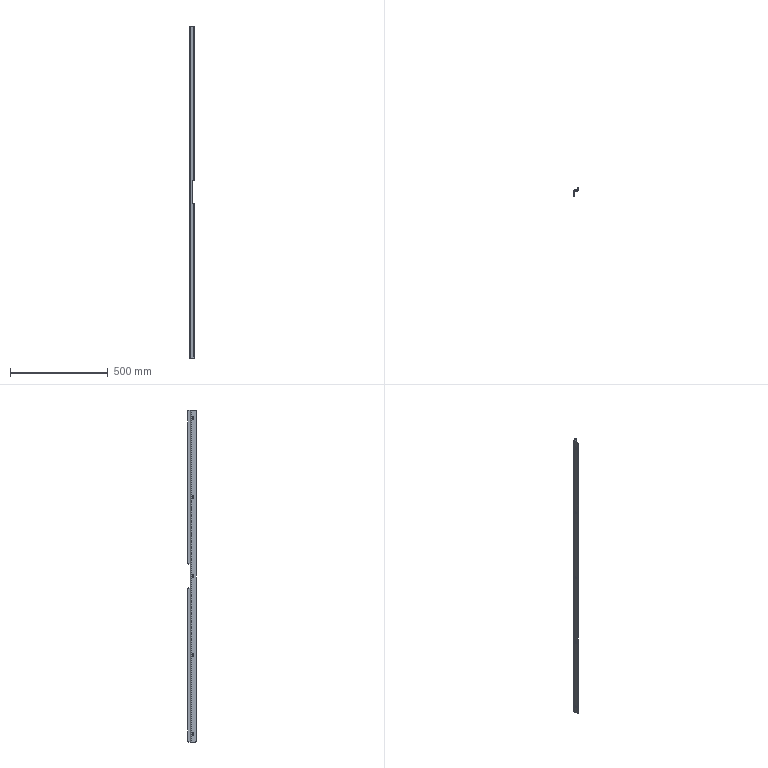Part | SolidWorks | features ICE 2, Fillet 1, FlatPattern 1, LPattern 1, SMBaseFlange 1, SheetMetal 1 | 1 solid | 60 faces | box 24 x 42 x 1700 mm | volume 301518 mm3 | plane 38 | cylinder 22 | commonest cylinder face diameters 7 x10 10 x6 2 x3 8 x3